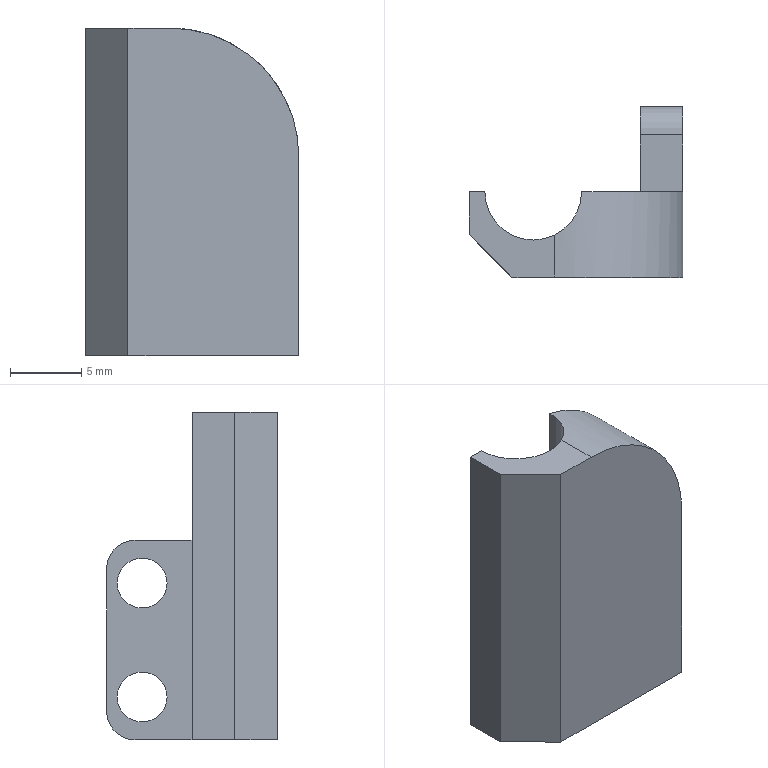Part | NX | features BREP 1 | 1 solid | 17 faces | box 15 x 12 x 23 mm | volume 1634 mm3 | plane 11 | cylinder 6 | commonest cylinder face diameters 3.5 x2 4 x2 6.8 x1 18 x1
STEP:
#1=CARTESIAN_POINT('',(3.,7.75,3.));
#2=VERTEX_POINT('',#1);
#3=CARTESIAN_POINT('',(3.,9.5,3.));
#4=DIRECTION('',(1.,0.,0.));
#5=DIRECTION('',(0.,-1.,0.));
#6=AXIS2_PLACEMENT_3D('',#3,#4,#5);
#7=CIRCLE('',#6,1.75);
#8=EDGE_CURVE('',#2,#2,#7,.T.);
#9=ORIENTED_EDGE('',*,*,#8,.T.);
#10=EDGE_LOOP('',(#9));
#11=FACE_BOUND('',#10,.T.);
#12=CARTESIAN_POINT('',(0.,11.25,3.));
#13=VERTEX_POINT('',#12);
#14=CARTESIAN_POINT('',(0.,9.5,3.));
#15=DIRECTION('',(1.,0.,0.));
#16=DIRECTION('',(0.,1.,0.));
#17=AXIS2_PLACEMENT_3D('',#14,#15,#16);
#18=CIRCLE('',#17,1.75);
#19=EDGE_CURVE('',#13,#13,#18,.T.);
#20=ORIENTED_EDGE('',*,*,#19,.F.);
#21=EDGE_LOOP('',(#20));
#22=FACE_BOUND('',#21,.T.);
#23=CARTESIAN_POINT('',(-10.,9.5,3.));
#24=DIRECTION('',(1.,0.,0.));
#25=DIRECTION('',(0.,1.,0.));
#26=AXIS2_PLACEMENT_3D('',#23,#24,#25);
#27=CYLINDRICAL_SURFACE('',#26,1.75);
#28=ADVANCED_FACE('',(#11,#22),#27,.F.);
#29=CARTESIAN_POINT('',(3.,11.25,11.));
#30=VERTEX_POINT('',#29);
#31=CARTESIAN_POINT('',(3.,9.5,11.));
#32=DIRECTION('',(1.,0.,0.));
#33=DIRECTION('',(0.,1.,0.));
#34=AXIS2_PLACEMENT_3D('',#31,#32,#33);
#35=CIRCLE('',#34,1.75);
#36=EDGE_CURVE('',#30,#30,#35,.T.);
#37=ORIENTED_EDGE('',*,*,#36,.T.);
#38=EDGE_LOOP('',(#37));
#39=FACE_BOUND('',#38,.T.);
#40=CARTESIAN_POINT('',(0.,11.25,11.));
#41=VERTEX_POINT('',#40);
#42=CARTESIAN_POINT('',(0.,9.5,11.));
#43=DIRECTION('',(1.,0.,0.));
#44=DIRECTION('',(0.,1.,0.));
#45=AXIS2_PLACEMENT_3D('',#42,#43,#44);
#46=CIRCLE('',#45,1.75);
#47=EDGE_CURVE('',#41,#41,#46,.T.);
#48=ORIENTED_EDGE('',*,*,#47,.F.);
#49=EDGE_LOOP('',(#48));
#50=FACE_BOUND('',#49,.T.);
#51=CARTESIAN_POINT('',(-10.,9.5,11.));
#52=DIRECTION('',(1.,0.,0.));
#53=DIRECTION('',(0.,1.,0.));
#54=AXIS2_PLACEMENT_3D('',#51,#52,#53);
#55=CYLINDRICAL_SURFACE('',#54,1.75);
#56=ADVANCED_FACE('',(#39,#50),#55,.F.);
#57=CARTESIAN_POINT('',(-10.9,6.,0.));
#58=VERTEX_POINT('',#57);
#59=CARTESIAN_POINT('',(-12.,6.,0.));
#60=VERTEX_POINT('',#59);
#61=CARTESIAN_POINT('',(-10.9,6.,0.));
#62=DIRECTION('',(-1.,0.,0.));
#63=VECTOR('',#62,1000.);
#64=LINE('',#61,#63);
#65=EDGE_CURVE('',#58,#60,#64,.T.);
#66=ORIENTED_EDGE('',*,*,#65,.T.);
#67=CARTESIAN_POINT('',(-12.,6.,23.));
#68=VERTEX_POINT('',#67);
#69=CARTESIAN_POINT('',(-12.,6.,23.));
#70=DIRECTION('',(0.,0.,-1.));
#71=VECTOR('',#70,1000.);
#72=LINE('',#69,#71);
#73=EDGE_CURVE('',#68,#60,#72,.T.);
#74=ORIENTED_EDGE('',*,*,#73,.F.);
#75=CARTESIAN_POINT('',(-10.9,6.,23.));
#76=VERTEX_POINT('',#75);
#77=CARTESIAN_POINT('',(-10.9,6.,23.));
#78=DIRECTION('',(-1.,0.,0.));
#79=VECTOR('',#78,1000.);
#80=LINE('',#77,#79);
#81=EDGE_CURVE('',#76,#68,#80,.T.);
#82=ORIENTED_EDGE('',*,*,#81,.F.);
#83=CARTESIAN_POINT('',(-10.9,6.,23.));
#84=DIRECTION('',(0.,0.,-1.));
#85=VECTOR('',#84,1000.);
#86=LINE('',#83,#85);
#87=EDGE_CURVE('',#76,#58,#86,.T.);
#88=ORIENTED_EDGE('',*,*,#87,.T.);
#89=EDGE_LOOP('',(#66,#74,#82,#88));
#90=FACE_BOUND('',#89,.T.);
#91=CARTESIAN_POINT('',(-10.9,6.,23.));
#92=DIRECTION('',(0.,-1.,0.));
#93=DIRECTION('',(1.,0.,0.));
#94=AXIS2_PLACEMENT_3D('',#91,#92,#93);
#95=PLANE('',#94);
#96=ADVANCED_FACE('',(#90),#95,.F.);
#97=CARTESIAN_POINT('',(-12.,3.,0.));
#98=VERTEX_POINT('',#97);
#99=CARTESIAN_POINT('',(-12.,6.,0.));
#100=DIRECTION('',(0.,-1.,0.));
#101=VECTOR('',#100,1000.);
#102=LINE('',#99,#101);
#103=EDGE_CURVE('',#60,#98,#102,.T.);
#104=ORIENTED_EDGE('',*,*,#103,.T.);
#105=CARTESIAN_POINT('',(-12.,3.,23.));
#106=VERTEX_POINT('',#105);
#107=CARTESIAN_POINT('',(-12.,3.,23.));
#108=DIRECTION('',(0.,0.,1.));
#109=VECTOR('',#108,1000.);
#110=LINE('',#107,#109);
#111=EDGE_CURVE('',#98,#106,#110,.T.);
#112=ORIENTED_EDGE('',*,*,#111,.T.);
#113=CARTESIAN_POINT('',(-12.,6.,23.));
#114=DIRECTION('',(0.,-1.,0.));
#115=VECTOR('',#114,1000.);
#116=LINE('',#113,#115);
#117=EDGE_CURVE('',#68,#106,#116,.T.);
#118=ORIENTED_EDGE('',*,*,#117,.F.);
#119=ORIENTED_EDGE('',*,*,#73,.T.);
#120=EDGE_LOOP('',(#104,#112,#118,#119));
#121=FACE_BOUND('',#120,.T.);
#122=CARTESIAN_POINT('',(-12.,6.,23.));
#123=DIRECTION('',(1.,0.,0.));
#124=DIRECTION('',(0.,0.,-1.));
#125=AXIS2_PLACEMENT_3D('',#122,#123,#124);
#126=PLANE('',#125);
#127=ADVANCED_FACE('',(#121),#126,.F.);
#128=CARTESIAN_POINT('',(3.,0.,14.));
#129=VERTEX_POINT('',#128);
#130=CARTESIAN_POINT('',(3.,0.,0.));
#131=VERTEX_POINT('',#130);
#132=CARTESIAN_POINT('',(3.,0.,23.));
#133=DIRECTION('',(0.,0.,-1.));
#134=VECTOR('',#133,1000.);
#135=LINE('',#132,#134);
#136=EDGE_CURVE('',#129,#131,#135,.T.);
#137=ORIENTED_EDGE('',*,*,#136,.F.);
#138=CARTESIAN_POINT('',(-6.,0.,23.));
#139=VERTEX_POINT('',#138);
#140=CARTESIAN_POINT('',(-6.,0.,14.));
#141=DIRECTION('',(0.,-1.,0.));
#142=DIRECTION('',(0.,0.,1.));
#143=AXIS2_PLACEMENT_3D('',#140,#141,#142);
#144=CIRCLE('',#143,9.);
#145=EDGE_CURVE('',#129,#139,#144,.T.);
#146=ORIENTED_EDGE('',*,*,#145,.T.);
#147=CARTESIAN_POINT('',(-9.,0.,23.));
#148=VERTEX_POINT('',#147);
#149=CARTESIAN_POINT('',(-12.,0.,23.));
#150=DIRECTION('',(1.,0.,0.));
#151=VECTOR('',#150,1000.);
#152=LINE('',#149,#151);
#153=EDGE_CURVE('',#148,#139,#152,.T.);
#154=ORIENTED_EDGE('',*,*,#153,.F.);
#155=CARTESIAN_POINT('',(-9.,0.,0.));
#156=VERTEX_POINT('',#155);
#157=CARTESIAN_POINT('',(-9.,0.,23.));
#158=DIRECTION('',(0.,0.,-1.));
#159=VECTOR('',#158,1000.);
#160=LINE('',#157,#159);
#161=EDGE_CURVE('',#148,#156,#160,.T.);
#162=ORIENTED_EDGE('',*,*,#161,.T.);
#163=CARTESIAN_POINT('',(-12.,0.,0.));
#164=DIRECTION('',(1.,0.,0.));
#165=VECTOR('',#164,1000.);
#166=LINE('',#163,#165);
#167=EDGE_CURVE('',#156,#131,#166,.T.);
#168=ORIENTED_EDGE('',*,*,#167,.T.);
#169=EDGE_LOOP('',(#137,#146,#154,#162,#168));
#170=FACE_BOUND('',#169,.T.);
#171=CARTESIAN_POINT('',(-12.,0.,23.));
#172=DIRECTION('',(0.,1.,0.));
#173=DIRECTION('',(0.,0.,1.));
#174=AXIS2_PLACEMENT_3D('',#171,#172,#173);
#175=PLANE('',#174);
#176=ADVANCED_FACE('',(#170),#175,.F.);
#177=ORIENTED_EDGE('',*,*,#8,.F.);
#178=EDGE_LOOP('',(#177));
#179=FACE_BOUND('',#178,.T.);
#180=ORIENTED_EDGE('',*,*,#36,.F.);
#181=EDGE_LOOP('',(#180));
#182=FACE_BOUND('',#181,.T.);
#183=CARTESIAN_POINT('',(3.,10.,0.));
#184=VERTEX_POINT('',#183);
#185=CARTESIAN_POINT('',(3.,0.,0.));
#186=DIRECTION('',(0.,1.,0.));
#187=VECTOR('',#186,1000.);
#188=LINE('',#185,#187);
#189=EDGE_CURVE('',#131,#184,#188,.T.);
#190=ORIENTED_EDGE('',*,*,#189,.T.);
#191=CARTESIAN_POINT('',(3.,12.,2.));
#192=VERTEX_POINT('',#191);
#193=CARTESIAN_POINT('',(3.,10.,2.));
#194=DIRECTION('',(1.,0.,0.));
#195=DIRECTION('',(0.,-1.,0.));
#196=AXIS2_PLACEMENT_3D('',#193,#194,#195);
#197=CIRCLE('',#196,2.);
#198=EDGE_CURVE('',#184,#192,#197,.T.);
#199=ORIENTED_EDGE('',*,*,#198,.T.);
#200=CARTESIAN_POINT('',(3.,12.,12.));
#201=VERTEX_POINT('',#200);
#202=CARTESIAN_POINT('',(3.,12.,23.));
#203=DIRECTION('',(0.,0.,-1.));
#204=VECTOR('',#203,1000.);
#205=LINE('',#202,#204);
#206=EDGE_CURVE('',#201,#192,#205,.T.);
#207=ORIENTED_EDGE('',*,*,#206,.F.);
#208=CARTESIAN_POINT('',(3.,10.,14.));
#209=VERTEX_POINT('',#208);
#210=CARTESIAN_POINT('',(3.,10.,12.));
#211=DIRECTION('',(1.,0.,0.));
#212=DIRECTION('',(0.,-1.,0.));
#213=AXIS2_PLACEMENT_3D('',#210,#211,#212);
#214=CIRCLE('',#213,2.);
#215=EDGE_CURVE('',#201,#209,#214,.T.);
#216=ORIENTED_EDGE('',*,*,#215,.T.);
#217=CARTESIAN_POINT('',(3.,6.,14.));
#218=VERTEX_POINT('',#217);
#219=CARTESIAN_POINT('',(3.,12.,14.));
#220=DIRECTION('',(0.,1.,0.));
#221=VECTOR('',#220,1000.);
#222=LINE('',#219,#221);
#223=EDGE_CURVE('',#218,#209,#222,.T.);
#224=ORIENTED_EDGE('',*,*,#223,.F.);
#225=CARTESIAN_POINT('',(3.,0.,14.));
#226=DIRECTION('',(0.,-1.,0.));
#227=VECTOR('',#226,1000.);
#228=LINE('',#225,#227);
#229=EDGE_CURVE('',#218,#129,#228,.T.);
#230=ORIENTED_EDGE('',*,*,#229,.T.);
#231=ORIENTED_EDGE('',*,*,#136,.T.);
#232=EDGE_LOOP('',(#190,#199,#207,#216,#224,#230,#231));
#233=FACE_BOUND('',#232,.T.);
#234=CARTESIAN_POINT('',(3.,0.,23.));
#235=DIRECTION('',(-1.,0.,0.));
#236=DIRECTION('',(0.,-1.,0.));
#237=AXIS2_PLACEMENT_3D('',#234,#235,#236);
#238=PLANE('',#237);
#239=ADVANCED_FACE('',(#179,#182,#233),#238,.F.);
#240=ORIENTED_EDGE('',*,*,#206,.T.);
#241=CARTESIAN_POINT('',(0.,12.,2.));
#242=VERTEX_POINT('',#241);
#243=CARTESIAN_POINT('',(3.,12.,2.));
#244=DIRECTION('',(-1.,0.,0.));
#245=VECTOR('',#244,1000.);
#246=LINE('',#243,#245);
#247=EDGE_CURVE('',#192,#242,#246,.T.);
#248=ORIENTED_EDGE('',*,*,#247,.T.);
#249=CARTESIAN_POINT('',(0.,12.,12.));
#250=VERTEX_POINT('',#249);
#251=CARTESIAN_POINT('',(0.,12.,23.));
#252=DIRECTION('',(0.,0.,-1.));
#253=VECTOR('',#252,1000.);
#254=LINE('',#251,#253);
#255=EDGE_CURVE('',#250,#242,#254,.T.);
#256=ORIENTED_EDGE('',*,*,#255,.F.);
#257=CARTESIAN_POINT('',(3.,12.,12.));
#258=DIRECTION('',(1.,0.,0.));
#259=VECTOR('',#258,1000.);
#260=LINE('',#257,#259);
#261=EDGE_CURVE('',#250,#201,#260,.T.);
#262=ORIENTED_EDGE('',*,*,#261,.T.);
#263=EDGE_LOOP('',(#240,#248,#256,#262));
#264=FACE_BOUND('',#263,.T.);
#265=CARTESIAN_POINT('',(3.,12.,23.));
#266=DIRECTION('',(0.,-1.,0.));
#267=DIRECTION('',(0.,0.,-1.));
#268=AXIS2_PLACEMENT_3D('',#265,#266,#267);
#269=PLANE('',#268);
#270=ADVANCED_FACE('',(#264),#269,.F.);
#271=ORIENTED_EDGE('',*,*,#19,.T.);
#272=EDGE_LOOP('',(#271));
#273=FACE_BOUND('',#272,.T.);
#274=ORIENTED_EDGE('',*,*,#47,.T.);
#275=EDGE_LOOP('',(#274));
#276=FACE_BOUND('',#275,.T.);
#277=ORIENTED_EDGE('',*,*,#255,.T.);
#278=CARTESIAN_POINT('',(0.,10.,0.));
#279=VERTEX_POINT('',#278);
#280=CARTESIAN_POINT('',(0.,10.,2.));
#281=DIRECTION('',(-1.,0.,0.));
#282=DIRECTION('',(0.,1.,0.));
#283=AXIS2_PLACEMENT_3D('',#280,#281,#282);
#284=CIRCLE('',#283,2.);
#285=EDGE_CURVE('',#242,#279,#284,.T.);
#286=ORIENTED_EDGE('',*,*,#285,.T.);
#287=CARTESIAN_POINT('',(0.,6.,0.));
#288=VERTEX_POINT('',#287);
#289=CARTESIAN_POINT('',(0.,12.,0.));
#290=DIRECTION('',(0.,-1.,0.));
#291=VECTOR('',#290,1000.);
#292=LINE('',#289,#291);
#293=EDGE_CURVE('',#279,#288,#292,.T.);
#294=ORIENTED_EDGE('',*,*,#293,.T.);
#295=CARTESIAN_POINT('',(0.,6.,14.));
#296=VERTEX_POINT('',#295);
#297=CARTESIAN_POINT('',(0.,6.,23.));
#298=DIRECTION('',(0.,0.,-1.));
#299=VECTOR('',#298,1000.);
#300=LINE('',#297,#299);
#301=EDGE_CURVE('',#296,#288,#300,.T.);
#302=ORIENTED_EDGE('',*,*,#301,.F.);
#303=CARTESIAN_POINT('',(0.,10.,14.));
#304=VERTEX_POINT('',#303);
#305=CARTESIAN_POINT('',(0.,12.,14.));
#306=DIRECTION('',(0.,1.,0.));
#307=VECTOR('',#306,1000.);
#308=LINE('',#305,#307);
#309=EDGE_CURVE('',#296,#304,#308,.T.);
#310=ORIENTED_EDGE('',*,*,#309,.T.);
#311=CARTESIAN_POINT('',(0.,10.,12.));
#312=DIRECTION('',(-1.,0.,0.));
#313=DIRECTION('',(0.,1.,0.));
#314=AXIS2_PLACEMENT_3D('',#311,#312,#313);
#315=CIRCLE('',#314,2.);
#316=EDGE_CURVE('',#304,#250,#315,.T.);
#317=ORIENTED_EDGE('',*,*,#316,.T.);
#318=EDGE_LOOP('',(#277,#286,#294,#302,#310,#317));
#319=FACE_BOUND('',#318,.T.);
#320=CARTESIAN_POINT('',(0.,12.,23.));
#321=DIRECTION('',(1.,0.,0.));
#322=DIRECTION('',(0.,1.,0.));
#323=AXIS2_PLACEMENT_3D('',#320,#321,#322);
#324=PLANE('',#323);
#325=ADVANCED_FACE('',(#273,#276,#319),#324,.F.);
#326=CARTESIAN_POINT('',(-4.1,6.,22.797));
#327=VERTEX_POINT('',#326);
#328=CARTESIAN_POINT('',(-4.1,6.,0.));
#329=VERTEX_POINT('',#328);
#330=CARTESIAN_POINT('',(-4.1,6.,23.));
#331=DIRECTION('',(0.,0.,-1.));
#332=VECTOR('',#331,1000.);
#333=LINE('',#330,#332);
#334=EDGE_CURVE('',#327,#329,#333,.T.);
#335=ORIENTED_EDGE('',*,*,#334,.F.);
#336=CARTESIAN_POINT('',(-6.,6.,14.));
#337=DIRECTION('',(0.,1.,0.));
#338=DIRECTION('',(0.,0.,-1.));
#339=AXIS2_PLACEMENT_3D('',#336,#337,#338);
#340=CIRCLE('',#339,9.);
#341=EDGE_CURVE('',#327,#218,#340,.T.);
#342=ORIENTED_EDGE('',*,*,#341,.T.);
#343=CARTESIAN_POINT('',(-10.,6.,14.));
#344=DIRECTION('',(1.,0.,0.));
#345=VECTOR('',#344,1000.);
#346=LINE('',#343,#345);
#347=EDGE_CURVE('',#296,#218,#346,.T.);
#348=ORIENTED_EDGE('',*,*,#347,.F.);
#349=ORIENTED_EDGE('',*,*,#301,.T.);
#350=CARTESIAN_POINT('',(0.,6.,0.));
#351=DIRECTION('',(-1.,0.,0.));
#352=VECTOR('',#351,1000.);
#353=LINE('',#350,#352);
#354=EDGE_CURVE('',#288,#329,#353,.T.);
#355=ORIENTED_EDGE('',*,*,#354,.T.);
#356=EDGE_LOOP('',(#335,#342,#348,#349,#355));
#357=FACE_BOUND('',#356,.T.);
#358=CARTESIAN_POINT('',(0.,6.,23.));
#359=DIRECTION('',(0.,-1.,0.));
#360=DIRECTION('',(0.,0.,-1.));
#361=AXIS2_PLACEMENT_3D('',#358,#359,#360);
#362=PLANE('',#361);
#363=ADVANCED_FACE('',(#357),#362,.F.);
#364=CARTESIAN_POINT('',(-6.,2.949,23.));
#365=VERTEX_POINT('',#364);
#366=CARTESIAN_POINT('',(-7.5,6.,23.));
#367=DIRECTION('',(0.,0.,-1.));
#368=DIRECTION('',(1.,0.,0.));
#369=AXIS2_PLACEMENT_3D('',#366,#367,#368);
#370=CIRCLE('',#369,3.4);
#371=EDGE_CURVE('',#365,#76,#370,.T.);
#372=ORIENTED_EDGE('',*,*,#371,.F.);
#373=CARTESIAN_POINT('',(-6.,2.949,23.));
#374=CARTESIAN_POINT('',(-4.855,3.512,23.));
#375=CARTESIAN_POINT('',(-4.1,4.724,22.797));
#376=CARTESIAN_POINT('',(-4.1,6.,22.797));
#377=B_SPLINE_CURVE_WITH_KNOTS('',3,(#373,#374,#375,#376),.UNSPECIFIED.,.F.,.F.,(4,4),(0.,0.003772),.UNSPECIFIED.);
#378=EDGE_CURVE('',#365,#327,#377,.T.);
#379=ORIENTED_EDGE('',*,*,#378,.T.);
#380=ORIENTED_EDGE('',*,*,#334,.T.);
#381=CARTESIAN_POINT('',(-7.5,6.,0.));
#382=DIRECTION('',(0.,0.,-1.));
#383=DIRECTION('',(1.,0.,0.));
#384=AXIS2_PLACEMENT_3D('',#381,#382,#383);
#385=CIRCLE('',#384,3.4);
#386=EDGE_CURVE('',#329,#58,#385,.T.);
#387=ORIENTED_EDGE('',*,*,#386,.T.);
#388=ORIENTED_EDGE('',*,*,#87,.F.);
#389=EDGE_LOOP('',(#372,#379,#380,#387,#388));
#390=FACE_BOUND('',#389,.T.);
#391=CARTESIAN_POINT('',(-7.5,6.,23.));
#392=DIRECTION('',(0.,0.,-1.));
#393=DIRECTION('',(-1.,0.,0.));
#394=AXIS2_PLACEMENT_3D('',#391,#392,#393);
#395=CYLINDRICAL_SURFACE('',#394,3.4);
#396=ADVANCED_FACE('',(#390),#395,.F.);
#397=ORIENTED_EDGE('',*,*,#153,.T.);
#398=CARTESIAN_POINT('',(-6.,6.,23.));
#399=DIRECTION('',(0.,1.,0.));
#400=VECTOR('',#399,1000.);
#401=LINE('',#398,#400);
#402=EDGE_CURVE('',#139,#365,#401,.T.);
#403=ORIENTED_EDGE('',*,*,#402,.T.);
#404=ORIENTED_EDGE('',*,*,#371,.T.);
#405=ORIENTED_EDGE('',*,*,#81,.T.);
#406=ORIENTED_EDGE('',*,*,#117,.T.);
#407=CARTESIAN_POINT('',(-11.25,2.25,23.));
#408=DIRECTION('',(0.7071,-0.7071,0.));
#409=VECTOR('',#408,1000.);
#410=LINE('',#407,#409);
#411=EDGE_CURVE('',#106,#148,#410,.T.);
#412=ORIENTED_EDGE('',*,*,#411,.T.);
#413=EDGE_LOOP('',(#397,#403,#404,#405,#406,#412));
#414=FACE_BOUND('',#413,.T.);
#415=CARTESIAN_POINT('',(-7.5,6.,23.));
#416=DIRECTION('',(0.,0.,1.));
#417=DIRECTION('',(1.,0.,0.));
#418=AXIS2_PLACEMENT_3D('',#415,#416,#417);
#419=PLANE('',#418);
#420=ADVANCED_FACE('',(#414),#419,.T.);
#421=ORIENTED_EDGE('',*,*,#293,.F.);
#422=CARTESIAN_POINT('',(-7.5,10.,0.));
#423=DIRECTION('',(1.,0.,0.));
#424=VECTOR('',#423,1000.);
#425=LINE('',#422,#424);
#426=EDGE_CURVE('',#279,#184,#425,.T.);
#427=ORIENTED_EDGE('',*,*,#426,.T.);
#428=ORIENTED_EDGE('',*,*,#189,.F.);
#429=ORIENTED_EDGE('',*,*,#167,.F.);
#430=CARTESIAN_POINT('',(-9.,0.,0.));
#431=DIRECTION('',(-0.7071,0.7071,0.));
#432=VECTOR('',#431,1000.);
#433=LINE('',#430,#432);
#434=EDGE_CURVE('',#156,#98,#433,.T.);
#435=ORIENTED_EDGE('',*,*,#434,.T.);
#436=ORIENTED_EDGE('',*,*,#103,.F.);
#437=ORIENTED_EDGE('',*,*,#65,.F.);
#438=ORIENTED_EDGE('',*,*,#386,.F.);
#439=ORIENTED_EDGE('',*,*,#354,.F.);
#440=EDGE_LOOP('',(#421,#427,#428,#429,#435,#436,#437,#438,#439));
#441=FACE_BOUND('',#440,.T.);
#442=CARTESIAN_POINT('',(-7.5,6.,0.));
#443=DIRECTION('',(0.,0.,1.));
#444=DIRECTION('',(1.,0.,0.));
#445=AXIS2_PLACEMENT_3D('',#442,#443,#444);
#446=PLANE('',#445);
#447=ADVANCED_FACE('',(#441),#446,.F.);
#448=ORIENTED_EDGE('',*,*,#411,.F.);
#449=ORIENTED_EDGE('',*,*,#111,.F.);
#450=ORIENTED_EDGE('',*,*,#434,.F.);
#451=ORIENTED_EDGE('',*,*,#161,.F.);
#452=EDGE_LOOP('',(#448,#449,#450,#451));
#453=FACE_BOUND('',#452,.T.);
#454=CARTESIAN_POINT('',(-9.,0.,23.));
#455=DIRECTION('',(0.7071,0.7071,0.));
#456=DIRECTION('',(0.,0.,-1.));
#457=AXIS2_PLACEMENT_3D('',#454,#455,#456);
#458=PLANE('',#457);
#459=ADVANCED_FACE('',(#453),#458,.F.);
#460=ORIENTED_EDGE('',*,*,#223,.T.);
#461=CARTESIAN_POINT('',(-10.,10.,14.));
#462=DIRECTION('',(-1.,0.,0.));
#463=VECTOR('',#462,1000.);
#464=LINE('',#461,#463);
#465=EDGE_CURVE('',#209,#304,#464,.T.);
#466=ORIENTED_EDGE('',*,*,#465,.T.);
#467=ORIENTED_EDGE('',*,*,#309,.F.);
#468=ORIENTED_EDGE('',*,*,#347,.T.);
#469=EDGE_LOOP('',(#460,#466,#467,#468));
#470=FACE_BOUND('',#469,.T.);
#471=CARTESIAN_POINT('',(-10.,12.,14.));
#472=DIRECTION('',(0.,0.,-1.));
#473=DIRECTION('',(-1.,0.,0.));
#474=AXIS2_PLACEMENT_3D('',#471,#472,#473);
#475=PLANE('',#474);
#476=ADVANCED_FACE('',(#470),#475,.F.);
#477=ORIENTED_EDGE('',*,*,#145,.F.);
#478=ORIENTED_EDGE('',*,*,#229,.F.);
#479=ORIENTED_EDGE('',*,*,#341,.F.);
#480=ORIENTED_EDGE('',*,*,#378,.F.);
#481=ORIENTED_EDGE('',*,*,#402,.F.);
#482=EDGE_LOOP('',(#477,#478,#479,#480,#481));
#483=FACE_BOUND('',#482,.T.);
#484=CARTESIAN_POINT('',(-6.,6.,14.));
#485=DIRECTION('',(0.,-1.,0.));
#486=DIRECTION('',(1.,0.,0.));
#487=AXIS2_PLACEMENT_3D('',#484,#485,#486);
#488=CYLINDRICAL_SURFACE('',#487,9.);
#489=ADVANCED_FACE('',(#483),#488,.T.);
#490=ORIENTED_EDGE('',*,*,#198,.F.);
#491=ORIENTED_EDGE('',*,*,#426,.F.);
#492=ORIENTED_EDGE('',*,*,#285,.F.);
#493=ORIENTED_EDGE('',*,*,#247,.F.);
#494=EDGE_LOOP('',(#490,#491,#492,#493));
#495=FACE_BOUND('',#494,.T.);
#496=CARTESIAN_POINT('',(3.,10.,2.));
#497=DIRECTION('',(-1.,0.,0.));
#498=DIRECTION('',(0.,0.,1.));
#499=AXIS2_PLACEMENT_3D('',#496,#497,#498);
#500=CYLINDRICAL_SURFACE('',#499,2.);
#501=ADVANCED_FACE('',(#495),#500,.T.);
#502=ORIENTED_EDGE('',*,*,#316,.F.);
#503=ORIENTED_EDGE('',*,*,#465,.F.);
#504=ORIENTED_EDGE('',*,*,#215,.F.);
#505=ORIENTED_EDGE('',*,*,#261,.F.);
#506=EDGE_LOOP('',(#502,#503,#504,#505));
#507=FACE_BOUND('',#506,.T.);
#508=CARTESIAN_POINT('',(3.,10.,12.));
#509=DIRECTION('',(1.,0.,0.));
#510=DIRECTION('',(0.,0.,-1.));
#511=AXIS2_PLACEMENT_3D('',#508,#509,#510);
#512=CYLINDRICAL_SURFACE('',#511,2.);
#513=ADVANCED_FACE('',(#507),#512,.T.);
#514=CLOSED_SHELL('',(#28,#56,#96,#127,#176,#239,#270,#325,#363,#396,#420,#447,#459,#476,#489,#501,#513));
#515=MANIFOLD_SOLID_BREP('',#514);
#516=(LENGTH_UNIT()NAMED_UNIT(*)SI_UNIT(.MILLI.,.METRE.));
#517=UNCERTAINTY_MEASURE_WITH_UNIT(LENGTH_MEASURE(0.0508),#516,'','');
#518=(NAMED_UNIT(*)PLANE_ANGLE_UNIT()SI_UNIT($,.RADIAN.));
#519=(NAMED_UNIT(*)SI_UNIT($,.STERADIAN.)SOLID_ANGLE_UNIT());
#520=(GEOMETRIC_REPRESENTATION_CONTEXT(3)GLOBAL_UNCERTAINTY_ASSIGNED_CONTEXT((#517))GLOBAL_UNIT_ASSIGNED_CONTEXT((#516,#518,#519))REPRESENTATION_CONTEXT('',''));
#521=ADVANCED_BREP_SHAPE_REPRESENTATION('',(#515),#520);